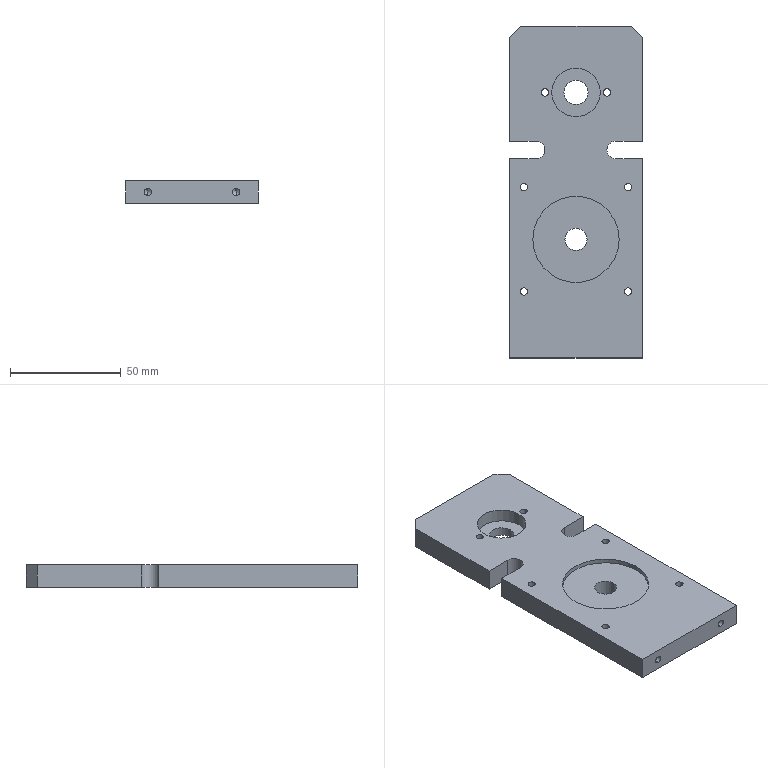Part | SolidWorks | features Cut 4, HoleWzd 3, Chamfer 1, Extrusion 1, ICE 1, MirrorPattern 1 | 1 solid | 47 faces | box 60 x 150 x 10 mm | volume 80933 mm3 | cylinder 27 | plane 16 | cone 4 | commonest cylinder face diameters 3.3 x16 8 x3 10 x2 11 x2 22 x2 39 x2
STEP:
#1=CARTESIAN_POINT('',(20.,-63.5,6.65));
#2=VERTEX_POINT('',#1);
#3=CARTESIAN_POINT('',(20.,-63.5,3.35));
#4=VERTEX_POINT('',#3);
#5=CARTESIAN_POINT('',(20.,-63.5,5.));
#6=DIRECTION('',(0.,-1.,0.));
#7=DIRECTION('',(0.,0.,-1.));
#8=AXIS2_PLACEMENT_3D('',#5,#6,#7);
#9=CIRCLE('',#8,1.65);
#10=EDGE_CURVE('',#2,#4,#9,.T.);
#11=ORIENTED_EDGE('',*,*,#10,.F.);
#12=CARTESIAN_POINT('',(20.,-75.,6.65));
#13=VERTEX_POINT('',#12);
#14=CARTESIAN_POINT('',(20.,-75.,6.65));
#15=DIRECTION('',(0.,-1.,0.));
#16=VECTOR('',#15,1000.);
#17=LINE('',#14,#16);
#18=EDGE_CURVE('',#2,#13,#17,.T.);
#19=ORIENTED_EDGE('',*,*,#18,.T.);
#20=CARTESIAN_POINT('',(20.,-75.,3.35));
#21=VERTEX_POINT('',#20);
#22=CARTESIAN_POINT('',(20.,-75.,5.));
#23=DIRECTION('',(0.,-1.,0.));
#24=DIRECTION('',(0.,0.,-1.));
#25=AXIS2_PLACEMENT_3D('',#22,#23,#24);
#26=CIRCLE('',#25,1.65);
#27=EDGE_CURVE('',#13,#21,#26,.T.);
#28=ORIENTED_EDGE('',*,*,#27,.T.);
#29=CARTESIAN_POINT('',(20.,-75.,3.35));
#30=DIRECTION('',(0.,-1.,0.));
#31=VECTOR('',#30,1000.);
#32=LINE('',#29,#31);
#33=EDGE_CURVE('',#4,#21,#32,.T.);
#34=ORIENTED_EDGE('',*,*,#33,.F.);
#35=EDGE_LOOP('',(#11,#19,#28,#34));
#36=FACE_OUTER_BOUND('',#35,.T.);
#37=CARTESIAN_POINT('',(20.,-75.,5.));
#38=DIRECTION('',(0.,-1.,0.));
#39=DIRECTION('',(0.,0.,-1.));
#40=AXIS2_PLACEMENT_3D('',#37,#38,#39);
#41=CYLINDRICAL_SURFACE('',#40,1.65);
#42=ADVANCED_FACE('',(#36),#41,.F.);
#43=CARTESIAN_POINT('',(20.,-62.509,5.));
#44=VERTEX_POINT('',#43);
#45=CARTESIAN_POINT('',(20.,-63.5,3.35));
#46=DIRECTION('',(0.,-0.515,-0.8572));
#47=VECTOR('',#46,1000.);
#48=LINE('',#45,#47);
#49=EDGE_CURVE('',#44,#4,#48,.T.);
#50=ORIENTED_EDGE('',*,*,#49,.F.);
#51=CARTESIAN_POINT('',(20.,-63.5,6.65));
#52=DIRECTION('',(0.,-0.515,0.8572));
#53=VECTOR('',#52,1000.);
#54=LINE('',#51,#53);
#55=EDGE_CURVE('',#44,#2,#54,.T.);
#56=ORIENTED_EDGE('',*,*,#55,.T.);
#57=ORIENTED_EDGE('',*,*,#10,.T.);
#58=EDGE_LOOP('',(#50,#56,#57));
#59=FACE_OUTER_BOUND('',#58,.T.);
#60=CARTESIAN_POINT('',(20.,-63.5,5.));
#61=DIRECTION('',(0.,-1.,0.));
#62=DIRECTION('',(0.,0.,-1.));
#63=AXIS2_PLACEMENT_3D('',#60,#61,#62);
#64=CONICAL_SURFACE('',#63,1.65,1.03);
#65=ADVANCED_FACE('',(#59),#64,.F.);
#66=CARTESIAN_POINT('',(-20.,-63.5,6.65));
#67=VERTEX_POINT('',#66);
#68=CARTESIAN_POINT('',(-20.,-63.5,3.35));
#69=VERTEX_POINT('',#68);
#70=CARTESIAN_POINT('',(-20.,-63.5,5.));
#71=DIRECTION('',(0.,-1.,0.));
#72=DIRECTION('',(0.,0.,-1.));
#73=AXIS2_PLACEMENT_3D('',#70,#71,#72);
#74=CIRCLE('',#73,1.65);
#75=EDGE_CURVE('',#67,#69,#74,.T.);
#76=ORIENTED_EDGE('',*,*,#75,.F.);
#77=CARTESIAN_POINT('',(-20.,-75.,6.65));
#78=VERTEX_POINT('',#77);
#79=CARTESIAN_POINT('',(-20.,-75.,6.65));
#80=DIRECTION('',(0.,-1.,0.));
#81=VECTOR('',#80,1000.);
#82=LINE('',#79,#81);
#83=EDGE_CURVE('',#67,#78,#82,.T.);
#84=ORIENTED_EDGE('',*,*,#83,.T.);
#85=CARTESIAN_POINT('',(-20.,-75.,3.35));
#86=VERTEX_POINT('',#85);
#87=CARTESIAN_POINT('',(-20.,-75.,5.));
#88=DIRECTION('',(0.,-1.,0.));
#89=DIRECTION('',(0.,0.,-1.));
#90=AXIS2_PLACEMENT_3D('',#87,#88,#89);
#91=CIRCLE('',#90,1.65);
#92=EDGE_CURVE('',#78,#86,#91,.T.);
#93=ORIENTED_EDGE('',*,*,#92,.T.);
#94=CARTESIAN_POINT('',(-20.,-75.,3.35));
#95=DIRECTION('',(0.,-1.,0.));
#96=VECTOR('',#95,1000.);
#97=LINE('',#94,#96);
#98=EDGE_CURVE('',#69,#86,#97,.T.);
#99=ORIENTED_EDGE('',*,*,#98,.F.);
#100=EDGE_LOOP('',(#76,#84,#93,#99));
#101=FACE_OUTER_BOUND('',#100,.T.);
#102=CARTESIAN_POINT('',(-20.,-75.,5.));
#103=DIRECTION('',(0.,-1.,0.));
#104=DIRECTION('',(0.,0.,-1.));
#105=AXIS2_PLACEMENT_3D('',#102,#103,#104);
#106=CYLINDRICAL_SURFACE('',#105,1.65);
#107=ADVANCED_FACE('',(#101),#106,.F.);
#108=CARTESIAN_POINT('',(-20.,-62.509,5.));
#109=VERTEX_POINT('',#108);
#110=CARTESIAN_POINT('',(-20.,-63.5,3.35));
#111=DIRECTION('',(0.,-0.515,-0.8572));
#112=VECTOR('',#111,1000.);
#113=LINE('',#110,#112);
#114=EDGE_CURVE('',#109,#69,#113,.T.);
#115=ORIENTED_EDGE('',*,*,#114,.F.);
#116=CARTESIAN_POINT('',(-20.,-63.5,6.65));
#117=DIRECTION('',(0.,-0.515,0.8572));
#118=VECTOR('',#117,1000.);
#119=LINE('',#116,#118);
#120=EDGE_CURVE('',#109,#67,#119,.T.);
#121=ORIENTED_EDGE('',*,*,#120,.T.);
#122=ORIENTED_EDGE('',*,*,#75,.T.);
#123=EDGE_LOOP('',(#115,#121,#122));
#124=FACE_OUTER_BOUND('',#123,.T.);
#125=CARTESIAN_POINT('',(-20.,-63.5,5.));
#126=DIRECTION('',(0.,-1.,0.));
#127=DIRECTION('',(0.,0.,-1.));
#128=AXIS2_PLACEMENT_3D('',#125,#126,#127);
#129=CONICAL_SURFACE('',#128,1.65,1.03);
#130=ADVANCED_FACE('',(#124),#129,.F.);
#131=CARTESIAN_POINT('',(-15.65,45.,0.));
#132=VERTEX_POINT('',#131);
#133=CARTESIAN_POINT('',(-12.35,45.,0.));
#134=VERTEX_POINT('',#133);
#135=CARTESIAN_POINT('',(-14.,45.,0.));
#136=DIRECTION('',(0.,0.,1.));
#137=DIRECTION('',(1.,0.,0.));
#138=AXIS2_PLACEMENT_3D('',#135,#136,#137);
#139=CIRCLE('',#138,1.65);
#140=EDGE_CURVE('',#132,#134,#139,.T.);
#141=ORIENTED_EDGE('',*,*,#140,.F.);
#142=CARTESIAN_POINT('',(-15.65,45.,10.));
#143=VERTEX_POINT('',#142);
#144=CARTESIAN_POINT('',(-15.65,45.,10.));
#145=DIRECTION('',(0.,0.,1.));
#146=VECTOR('',#145,1000.);
#147=LINE('',#144,#146);
#148=EDGE_CURVE('',#132,#143,#147,.T.);
#149=ORIENTED_EDGE('',*,*,#148,.T.);
#150=CARTESIAN_POINT('',(-12.35,45.,10.));
#151=VERTEX_POINT('',#150);
#152=CARTESIAN_POINT('',(-14.,45.,10.));
#153=DIRECTION('',(0.,0.,1.));
#154=DIRECTION('',(1.,0.,0.));
#155=AXIS2_PLACEMENT_3D('',#152,#153,#154);
#156=CIRCLE('',#155,1.65);
#157=EDGE_CURVE('',#143,#151,#156,.T.);
#158=ORIENTED_EDGE('',*,*,#157,.T.);
#159=CARTESIAN_POINT('',(-12.35,45.,10.));
#160=DIRECTION('',(0.,0.,1.));
#161=VECTOR('',#160,1000.);
#162=LINE('',#159,#161);
#163=EDGE_CURVE('',#134,#151,#162,.T.);
#164=ORIENTED_EDGE('',*,*,#163,.F.);
#165=EDGE_LOOP('',(#141,#149,#158,#164));
#166=FACE_OUTER_BOUND('',#165,.T.);
#167=CARTESIAN_POINT('',(-14.,45.,10.));
#168=DIRECTION('',(0.,0.,1.));
#169=DIRECTION('',(1.,0.,0.));
#170=AXIS2_PLACEMENT_3D('',#167,#168,#169);
#171=CYLINDRICAL_SURFACE('',#170,1.65);
#172=ADVANCED_FACE('',(#166),#171,.F.);
#173=CARTESIAN_POINT('',(12.35,45.,0.));
#174=VERTEX_POINT('',#173);
#175=CARTESIAN_POINT('',(15.65,45.,0.));
#176=VERTEX_POINT('',#175);
#177=CARTESIAN_POINT('',(14.,45.,0.));
#178=DIRECTION('',(0.,0.,1.));
#179=DIRECTION('',(1.,0.,0.));
#180=AXIS2_PLACEMENT_3D('',#177,#178,#179);
#181=CIRCLE('',#180,1.65);
#182=EDGE_CURVE('',#174,#176,#181,.T.);
#183=ORIENTED_EDGE('',*,*,#182,.F.);
#184=CARTESIAN_POINT('',(12.35,45.,10.));
#185=VERTEX_POINT('',#184);
#186=CARTESIAN_POINT('',(12.35,45.,10.));
#187=DIRECTION('',(0.,0.,1.));
#188=VECTOR('',#187,1000.);
#189=LINE('',#186,#188);
#190=EDGE_CURVE('',#174,#185,#189,.T.);
#191=ORIENTED_EDGE('',*,*,#190,.T.);
#192=CARTESIAN_POINT('',(15.65,45.,10.));
#193=VERTEX_POINT('',#192);
#194=CARTESIAN_POINT('',(14.,45.,10.));
#195=DIRECTION('',(0.,0.,1.));
#196=DIRECTION('',(1.,0.,0.));
#197=AXIS2_PLACEMENT_3D('',#194,#195,#196);
#198=CIRCLE('',#197,1.65);
#199=EDGE_CURVE('',#185,#193,#198,.T.);
#200=ORIENTED_EDGE('',*,*,#199,.T.);
#201=CARTESIAN_POINT('',(15.65,45.,10.));
#202=DIRECTION('',(0.,0.,1.));
#203=VECTOR('',#202,1000.);
#204=LINE('',#201,#203);
#205=EDGE_CURVE('',#176,#193,#204,.T.);
#206=ORIENTED_EDGE('',*,*,#205,.F.);
#207=EDGE_LOOP('',(#183,#191,#200,#206));
#208=FACE_OUTER_BOUND('',#207,.T.);
#209=CARTESIAN_POINT('',(14.,45.,10.));
#210=DIRECTION('',(0.,0.,1.));
#211=DIRECTION('',(1.,0.,0.));
#212=AXIS2_PLACEMENT_3D('',#209,#210,#211);
#213=CYLINDRICAL_SURFACE('',#212,1.65);
#214=ADVANCED_FACE('',(#208),#213,.F.);
#215=CARTESIAN_POINT('',(18.,23.,10.));
#216=VERTEX_POINT('',#215);
#217=CARTESIAN_POINT('',(14.,19.,10.));
#218=VERTEX_POINT('',#217);
#219=CARTESIAN_POINT('',(18.,19.,10.));
#220=DIRECTION('',(0.,0.,1.));
#221=DIRECTION('',(1.,0.,0.));
#222=AXIS2_PLACEMENT_3D('',#219,#220,#221);
#223=CIRCLE('',#222,4.);
#224=EDGE_CURVE('',#216,#218,#223,.T.);
#225=ORIENTED_EDGE('',*,*,#224,.T.);
#226=CARTESIAN_POINT('',(14.,19.,0.));
#227=VERTEX_POINT('',#226);
#228=CARTESIAN_POINT('',(14.,19.,10.));
#229=DIRECTION('',(0.,0.,-1.));
#230=VECTOR('',#229,1000.);
#231=LINE('',#228,#230);
#232=EDGE_CURVE('',#218,#227,#231,.T.);
#233=ORIENTED_EDGE('',*,*,#232,.T.);
#234=CARTESIAN_POINT('',(18.,23.,0.));
#235=VERTEX_POINT('',#234);
#236=CARTESIAN_POINT('',(18.,19.,0.));
#237=DIRECTION('',(0.,0.,1.));
#238=DIRECTION('',(1.,0.,0.));
#239=AXIS2_PLACEMENT_3D('',#236,#237,#238);
#240=CIRCLE('',#239,4.);
#241=EDGE_CURVE('',#235,#227,#240,.T.);
#242=ORIENTED_EDGE('',*,*,#241,.F.);
#243=CARTESIAN_POINT('',(18.,23.,10.));
#244=DIRECTION('',(0.,0.,-1.));
#245=VECTOR('',#244,1000.);
#246=LINE('',#243,#245);
#247=EDGE_CURVE('',#216,#235,#246,.T.);
#248=ORIENTED_EDGE('',*,*,#247,.F.);
#249=EDGE_LOOP('',(#225,#233,#242,#248));
#250=FACE_OUTER_BOUND('',#249,.T.);
#251=CARTESIAN_POINT('',(18.,19.,10.));
#252=DIRECTION('',(0.,0.,-1.));
#253=DIRECTION('',(-1.,0.,0.));
#254=AXIS2_PLACEMENT_3D('',#251,#252,#253);
#255=CYLINDRICAL_SURFACE('',#254,4.);
#256=ADVANCED_FACE('',(#250),#255,.F.);
#257=CARTESIAN_POINT('',(-5.5,45.,0.));
#258=VERTEX_POINT('',#257);
#259=CARTESIAN_POINT('',(5.5,45.,0.));
#260=VERTEX_POINT('',#259);
#261=CARTESIAN_POINT('',(0.,45.,0.));
#262=DIRECTION('',(0.,0.,1.));
#263=DIRECTION('',(1.,0.,0.));
#264=AXIS2_PLACEMENT_3D('',#261,#262,#263);
#265=CIRCLE('',#264,5.5);
#266=EDGE_CURVE('',#258,#260,#265,.T.);
#267=ORIENTED_EDGE('',*,*,#266,.F.);
#268=CARTESIAN_POINT('',(-5.5,45.,4.));
#269=VERTEX_POINT('',#268);
#270=CARTESIAN_POINT('',(-5.5,45.,0.));
#271=DIRECTION('',(0.,0.,1.));
#272=VECTOR('',#271,1000.);
#273=LINE('',#270,#272);
#274=EDGE_CURVE('',#258,#269,#273,.T.);
#275=ORIENTED_EDGE('',*,*,#274,.T.);
#276=CARTESIAN_POINT('',(5.5,45.,4.));
#277=VERTEX_POINT('',#276);
#278=CARTESIAN_POINT('',(0.,45.,4.));
#279=DIRECTION('',(0.,0.,1.));
#280=DIRECTION('',(1.,0.,0.));
#281=AXIS2_PLACEMENT_3D('',#278,#279,#280);
#282=CIRCLE('',#281,5.5);
#283=EDGE_CURVE('',#269,#277,#282,.T.);
#284=ORIENTED_EDGE('',*,*,#283,.T.);
#285=CARTESIAN_POINT('',(5.5,45.,0.));
#286=DIRECTION('',(0.,0.,1.));
#287=VECTOR('',#286,1000.);
#288=LINE('',#285,#287);
#289=EDGE_CURVE('',#260,#277,#288,.T.);
#290=ORIENTED_EDGE('',*,*,#289,.F.);
#291=EDGE_LOOP('',(#267,#275,#284,#290));
#292=FACE_OUTER_BOUND('',#291,.T.);
#293=CARTESIAN_POINT('',(0.,45.,0.));
#294=DIRECTION('',(0.,0.,1.));
#295=DIRECTION('',(1.,0.,0.));
#296=AXIS2_PLACEMENT_3D('',#293,#294,#295);
#297=CYLINDRICAL_SURFACE('',#296,5.5);
#298=ADVANCED_FACE('',(#292),#297,.F.);
#299=CARTESIAN_POINT('',(-11.,45.,4.));
#300=VERTEX_POINT('',#299);
#301=CARTESIAN_POINT('',(11.,45.,4.));
#302=VERTEX_POINT('',#301);
#303=CARTESIAN_POINT('',(0.,45.,4.));
#304=DIRECTION('',(0.,0.,1.));
#305=DIRECTION('',(1.,0.,0.));
#306=AXIS2_PLACEMENT_3D('',#303,#304,#305);
#307=CIRCLE('',#306,11.);
#308=EDGE_CURVE('',#300,#302,#307,.T.);
#309=ORIENTED_EDGE('',*,*,#308,.F.);
#310=CARTESIAN_POINT('',(-11.,45.,10.));
#311=VERTEX_POINT('',#310);
#312=CARTESIAN_POINT('',(-11.,45.,4.));
#313=DIRECTION('',(0.,0.,1.));
#314=VECTOR('',#313,1000.);
#315=LINE('',#312,#314);
#316=EDGE_CURVE('',#300,#311,#315,.T.);
#317=ORIENTED_EDGE('',*,*,#316,.T.);
#318=CARTESIAN_POINT('',(11.,45.,10.));
#319=VERTEX_POINT('',#318);
#320=CARTESIAN_POINT('',(0.,45.,10.));
#321=DIRECTION('',(0.,0.,1.));
#322=DIRECTION('',(1.,0.,0.));
#323=AXIS2_PLACEMENT_3D('',#320,#321,#322);
#324=CIRCLE('',#323,11.);
#325=EDGE_CURVE('',#311,#319,#324,.T.);
#326=ORIENTED_EDGE('',*,*,#325,.T.);
#327=CARTESIAN_POINT('',(11.,45.,4.));
#328=DIRECTION('',(0.,0.,1.));
#329=VECTOR('',#328,1000.);
#330=LINE('',#327,#329);
#331=EDGE_CURVE('',#302,#319,#330,.T.);
#332=ORIENTED_EDGE('',*,*,#331,.F.);
#333=EDGE_LOOP('',(#309,#317,#326,#332));
#334=FACE_OUTER_BOUND('',#333,.T.);
#335=CARTESIAN_POINT('',(0.,45.,4.));
#336=DIRECTION('',(0.,0.,1.));
#337=DIRECTION('',(1.,0.,0.));
#338=AXIS2_PLACEMENT_3D('',#335,#336,#337);
#339=CYLINDRICAL_SURFACE('',#338,11.);
#340=ADVANCED_FACE('',(#334),#339,.F.);
#341=CARTESIAN_POINT('',(-25.22,2.145,0.));
#342=VERTEX_POINT('',#341);
#343=CARTESIAN_POINT('',(-21.92,2.145,0.));
#344=VERTEX_POINT('',#343);
#345=CARTESIAN_POINT('',(-23.57,2.145,0.));
#346=DIRECTION('',(0.,0.,1.));
#347=DIRECTION('',(1.,0.,0.));
#348=AXIS2_PLACEMENT_3D('',#345,#346,#347);
#349=CIRCLE('',#348,1.65);
#350=EDGE_CURVE('',#342,#344,#349,.T.);
#351=ORIENTED_EDGE('',*,*,#350,.F.);
#352=CARTESIAN_POINT('',(-25.22,2.145,10.));
#353=VERTEX_POINT('',#352);
#354=CARTESIAN_POINT('',(-25.22,2.145,10.));
#355=DIRECTION('',(0.,0.,1.));
#356=VECTOR('',#355,1000.);
#357=LINE('',#354,#356);
#358=EDGE_CURVE('',#342,#353,#357,.T.);
#359=ORIENTED_EDGE('',*,*,#358,.T.);
#360=CARTESIAN_POINT('',(-21.92,2.145,10.));
#361=VERTEX_POINT('',#360);
#362=CARTESIAN_POINT('',(-23.57,2.145,10.));
#363=DIRECTION('',(0.,0.,1.));
#364=DIRECTION('',(1.,0.,0.));
#365=AXIS2_PLACEMENT_3D('',#362,#363,#364);
#366=CIRCLE('',#365,1.65);
#367=EDGE_CURVE('',#353,#361,#366,.T.);
#368=ORIENTED_EDGE('',*,*,#367,.T.);
#369=CARTESIAN_POINT('',(-21.92,2.145,10.));
#370=DIRECTION('',(0.,0.,1.));
#371=VECTOR('',#370,1000.);
#372=LINE('',#369,#371);
#373=EDGE_CURVE('',#344,#361,#372,.T.);
#374=ORIENTED_EDGE('',*,*,#373,.F.);
#375=EDGE_LOOP('',(#351,#359,#368,#374));
#376=FACE_OUTER_BOUND('',#375,.T.);
#377=CARTESIAN_POINT('',(-23.57,2.145,10.));
#378=DIRECTION('',(0.,0.,1.));
#379=DIRECTION('',(1.,0.,0.));
#380=AXIS2_PLACEMENT_3D('',#377,#378,#379);
#381=CYLINDRICAL_SURFACE('',#380,1.65);
#382=ADVANCED_FACE('',(#376),#381,.F.);
#383=CARTESIAN_POINT('',(-25.22,-44.995,0.));
#384=VERTEX_POINT('',#383);
#385=CARTESIAN_POINT('',(-21.92,-44.995,0.));
#386=VERTEX_POINT('',#385);
#387=CARTESIAN_POINT('',(-23.57,-44.995,0.));
#388=DIRECTION('',(0.,0.,1.));
#389=DIRECTION('',(1.,0.,0.));
#390=AXIS2_PLACEMENT_3D('',#387,#388,#389);
#391=CIRCLE('',#390,1.65);
#392=EDGE_CURVE('',#384,#386,#391,.T.);
#393=ORIENTED_EDGE('',*,*,#392,.F.);
#394=CARTESIAN_POINT('',(-25.22,-44.995,10.));
#395=VERTEX_POINT('',#394);
#396=CARTESIAN_POINT('',(-25.22,-44.995,10.));
#397=DIRECTION('',(0.,0.,1.));
#398=VECTOR('',#397,1000.);
#399=LINE('',#396,#398);
#400=EDGE_CURVE('',#384,#395,#399,.T.);
#401=ORIENTED_EDGE('',*,*,#400,.T.);
#402=CARTESIAN_POINT('',(-21.92,-44.995,10.));
#403=VERTEX_POINT('',#402);
#404=CARTESIAN_POINT('',(-23.57,-44.995,10.));
#405=DIRECTION('',(0.,0.,1.));
#406=DIRECTION('',(1.,0.,0.));
#407=AXIS2_PLACEMENT_3D('',#404,#405,#406);
#408=CIRCLE('',#407,1.65);
#409=EDGE_CURVE('',#395,#403,#408,.T.);
#410=ORIENTED_EDGE('',*,*,#409,.T.);
#411=CARTESIAN_POINT('',(-21.92,-44.995,10.));
#412=DIRECTION('',(0.,0.,1.));
#413=VECTOR('',#412,1000.);
#414=LINE('',#411,#413);
#415=EDGE_CURVE('',#386,#403,#414,.T.);
#416=ORIENTED_EDGE('',*,*,#415,.F.);
#417=EDGE_LOOP('',(#393,#401,#410,#416));
#418=FACE_OUTER_BOUND('',#417,.T.);
#419=CARTESIAN_POINT('',(-23.57,-44.995,10.));
#420=DIRECTION('',(0.,0.,1.));
#421=DIRECTION('',(1.,0.,0.));
#422=AXIS2_PLACEMENT_3D('',#419,#420,#421);
#423=CYLINDRICAL_SURFACE('',#422,1.65);
#424=ADVANCED_FACE('',(#418),#423,.F.);
#425=CARTESIAN_POINT('',(21.92,2.145,0.));
#426=VERTEX_POINT('',#425);
#427=CARTESIAN_POINT('',(25.22,2.145,0.));
#428=VERTEX_POINT('',#427);
#429=CARTESIAN_POINT('',(23.57,2.145,0.));
#430=DIRECTION('',(0.,0.,1.));
#431=DIRECTION('',(1.,0.,0.));
#432=AXIS2_PLACEMENT_3D('',#429,#430,#431);
#433=CIRCLE('',#432,1.65);
#434=EDGE_CURVE('',#426,#428,#433,.T.);
#435=ORIENTED_EDGE('',*,*,#434,.F.);
#436=CARTESIAN_POINT('',(21.92,2.145,10.));
#437=VERTEX_POINT('',#436);
#438=CARTESIAN_POINT('',(21.92,2.145,10.));
#439=DIRECTION('',(0.,0.,1.));
#440=VECTOR('',#439,1000.);
#441=LINE('',#438,#440);
#442=EDGE_CURVE('',#426,#437,#441,.T.);
#443=ORIENTED_EDGE('',*,*,#442,.T.);
#444=CARTESIAN_POINT('',(25.22,2.145,10.));
#445=VERTEX_POINT('',#444);
#446=CARTESIAN_POINT('',(23.57,2.145,10.));
#447=DIRECTION('',(0.,0.,1.));
#448=DIRECTION('',(1.,0.,0.));
#449=AXIS2_PLACEMENT_3D('',#446,#447,#448);
#450=CIRCLE('',#449,1.65);
#451=EDGE_CURVE('',#437,#445,#450,.T.);
#452=ORIENTED_EDGE('',*,*,#451,.T.);
#453=CARTESIAN_POINT('',(25.22,2.145,10.));
#454=DIRECTION('',(0.,0.,1.));
#455=VECTOR('',#454,1000.);
#456=LINE('',#453,#455);
#457=EDGE_CURVE('',#428,#445,#456,.T.);
#458=ORIENTED_EDGE('',*,*,#457,.F.);
#459=EDGE_LOOP('',(#435,#443,#452,#458));
#460=FACE_OUTER_BOUND('',#459,.T.);
#461=CARTESIAN_POINT('',(23.57,2.145,10.));
#462=DIRECTION('',(0.,0.,1.));
#463=DIRECTION('',(1.,0.,0.));
#464=AXIS2_PLACEMENT_3D('',#461,#462,#463);
#465=CYLINDRICAL_SURFACE('',#464,1.65);
#466=ADVANCED_FACE('',(#460),#465,.F.);
#467=CARTESIAN_POINT('',(21.92,-44.995,0.));
#468=VERTEX_POINT('',#467);
#469=CARTESIAN_POINT('',(25.22,-44.995,0.));
#470=VERTEX_POINT('',#469);
#471=CARTESIAN_POINT('',(23.57,-44.995,0.));
#472=DIRECTION('',(0.,0.,1.));
#473=DIRECTION('',(1.,0.,0.));
#474=AXIS2_PLACEMENT_3D('',#471,#472,#473);
#475=CIRCLE('',#474,1.65);
#476=EDGE_CURVE('',#468,#470,#475,.T.);
#477=ORIENTED_EDGE('',*,*,#476,.F.);
#478=CARTESIAN_POINT('',(21.92,-44.995,10.));
#479=VERTEX_POINT('',#478);
#480=CARTESIAN_POINT('',(21.92,-44.995,10.));
#481=DIRECTION('',(0.,0.,1.));
#482=VECTOR('',#481,1000.);
#483=LINE('',#480,#482);
#484=EDGE_CURVE('',#468,#479,#483,.T.);
#485=ORIENTED_EDGE('',*,*,#484,.T.);
#486=CARTESIAN_POINT('',(25.22,-44.995,10.));
#487=VERTEX_POINT('',#486);
#488=CARTESIAN_POINT('',(23.57,-44.995,10.));
#489=DIRECTION('',(0.,0.,1.));
#490=DIRECTION('',(1.,0.,0.));
#491=AXIS2_PLACEMENT_3D('',#488,#489,#490);
#492=CIRCLE('',#491,1.65);
#493=EDGE_CURVE('',#479,#487,#492,.T.);
#494=ORIENTED_EDGE('',*,*,#493,.T.);
#495=CARTESIAN_POINT('',(25.22,-44.995,10.));
#496=DIRECTION('',(0.,0.,1.));
#497=VECTOR('',#496,1000.);
#498=LINE('',#495,#497);
#499=EDGE_CURVE('',#470,#487,#498,.T.);
#500=ORIENTED_EDGE('',*,*,#499,.F.);
#501=EDGE_LOOP('',(#477,#485,#494,#500));
#502=FACE_OUTER_BOUND('',#501,.T.);
#503=CARTESIAN_POINT('',(23.57,-44.995,10.));
#504=DIRECTION('',(0.,0.,1.));
#505=DIRECTION('',(1.,0.,0.));
#506=AXIS2_PLACEMENT_3D('',#503,#504,#505);
#507=CYLINDRICAL_SURFACE('',#506,1.65);
#508=ADVANCED_FACE('',(#502),#507,.F.);
#509=CARTESIAN_POINT('',(-5.,-21.425,0.));
#510=VERTEX_POINT('',#509);
#511=CARTESIAN_POINT('',(5.,-21.425,0.));
#512=VERTEX_POINT('',#511);
#513=CARTESIAN_POINT('',(0.,-21.425,0.));
#514=DIRECTION('',(0.,0.,1.));
#515=DIRECTION('',(1.,0.,0.));
#516=AXIS2_PLACEMENT_3D('',#513,#514,#515);
#517=CIRCLE('',#516,5.);
#518=EDGE_CURVE('',#510,#512,#517,.T.);
#519=ORIENTED_EDGE('',*,*,#518,.F.);
#520=CARTESIAN_POINT('',(-5.,-21.425,8.));
#521=VERTEX_POINT('',#520);
#522=CARTESIAN_POINT('',(-5.,-21.425,0.));
#523=DIRECTION('',(0.,0.,1.));
#524=VECTOR('',#523,1000.);
#525=LINE('',#522,#524);
#526=EDGE_CURVE('',#510,#521,#525,.T.);
#527=ORIENTED_EDGE('',*,*,#526,.T.);
#528=CARTESIAN_POINT('',(5.,-21.425,8.));
#529=VERTEX_POINT('',#528);
#530=CARTESIAN_POINT('',(0.,-21.425,8.));
#531=DIRECTION('',(0.,0.,1.));
#532=DIRECTION('',(1.,0.,0.));
#533=AXIS2_PLACEMENT_3D('',#530,#531,#532);
#534=CIRCLE('',#533,5.);
#535=EDGE_CURVE('',#521,#529,#534,.T.);
#536=ORIENTED_EDGE('',*,*,#535,.T.);
#537=CARTESIAN_POINT('',(5.,-21.425,0.));
#538=DIRECTION('',(0.,0.,1.));
#539=VECTOR('',#538,1000.);
#540=LINE('',#537,#539);
#541=EDGE_CURVE('',#512,#529,#540,.T.);
#542=ORIENTED_EDGE('',*,*,#541,.F.);
#543=EDGE_LOOP('',(#519,#527,#536,#542));
#544=FACE_OUTER_BOUND('',#543,.T.);
#545=CARTESIAN_POINT('',(0.,-21.425,0.));
#546=DIRECTION('',(0.,0.,1.));
#547=DIRECTION('',(1.,0.,0.));
#548=AXIS2_PLACEMENT_3D('',#545,#546,#547);
#549=CYLINDRICAL_SURFACE('',#548,5.);
#550=ADVANCED_FACE('',(#544),#549,.F.);
#551=CARTESIAN_POINT('',(19.5,-21.425,8.));
#552=VERTEX_POINT('',#551);
#553=CARTESIAN_POINT('',(-19.5,-21.425,8.));
#554=VERTEX_POINT('',#553);
#555=CARTESIAN_POINT('',(0.,-21.425,8.));
#556=DIRECTION('',(0.,0.,-1.));
#557=DIRECTION('',(-1.,0.,0.));
#558=AXIS2_PLACEMENT_3D('',#555,#556,#557);
#559=CIRCLE('',#558,19.5);
#560=EDGE_CURVE('',#552,#554,#559,.T.);
#561=ORIENTED_EDGE('',*,*,#560,.T.);
#562=CARTESIAN_POINT('',(-19.5,-21.425,10.));
#563=VERTEX_POINT('',#562);
#564=CARTESIAN_POINT('',(-19.5,-21.425,8.));
#565=DIRECTION('',(0.,0.,1.));
#566=VECTOR('',#565,1000.);
#567=LINE('',#564,#566);
#568=EDGE_CURVE('',#554,#563,#567,.T.);
#569=ORIENTED_EDGE('',*,*,#568,.T.);
#570=CARTESIAN_POINT('',(19.5,-21.425,10.));
#571=VERTEX_POINT('',#570);
#572=CARTESIAN_POINT('',(0.,-21.425,10.));
#573=DIRECTION('',(0.,0.,-1.));
#574=DIRECTION('',(-1.,0.,0.));
#575=AXIS2_PLACEMENT_3D('',#572,#573,#574);
#576=CIRCLE('',#575,19.5);
#577=EDGE_CURVE('',#571,#563,#576,.T.);
#578=ORIENTED_EDGE('',*,*,#577,.F.);
#579=CARTESIAN_POINT('',(19.5,-21.425,8.));
#580=DIRECTION('',(0.,0.,1.));
#581=VECTOR('',#580,1000.);
#582=LINE('',#579,#581);
#583=EDGE_CURVE('',#552,#571,#582,.T.);
#584=ORIENTED_EDGE('',*,*,#583,.F.);
#585=EDGE_LOOP('',(#561,#569,#578,#584));
#586=FACE_OUTER_BOUND('',#585,.T.);
#587=CARTESIAN_POINT('',(0.,-21.425,8.));
#588=DIRECTION('',(0.,0.,1.));
#589=DIRECTION('',(1.,0.,0.));
#590=AXIS2_PLACEMENT_3D('',#587,#588,#589);
#591=CYLINDRICAL_SURFACE('',#590,19.5);
#592=ADVANCED_FACE('',(#586),#591,.F.);
#593=CARTESIAN_POINT('',(30.,15.,10.));
#594=VERTEX_POINT('',#593);
#595=CARTESIAN_POINT('',(30.,15.,0.));
#596=VERTEX_POINT('',#595);
#597=CARTESIAN_POINT('',(30.,15.,10.));
#598=DIRECTION('',(0.,0.,-1.));
#599=VECTOR('',#598,1000.);
#600=LINE('',#597,#599);
#601=EDGE_CURVE('',#594,#596,#600,.T.);
#602=ORIENTED_EDGE('',*,*,#601,.F.);
#603=CARTESIAN_POINT('',(30.,-75.,10.));
#604=VERTEX_POINT('',#603);
#605=CARTESIAN_POINT('',(30.,75.,10.));
#606=DIRECTION('',(0.,1.,0.));
#607=VECTOR('',#606,1000.);
#608=LINE('',#605,#607);
#609=EDGE_CURVE('',#604,#594,#608,.T.);
#610=ORIENTED_EDGE('',*,*,#609,.F.);
#611=CARTESIAN_POINT('',(30.,-75.,0.));
#612=VERTEX_POINT('',#611);
#613=CARTESIAN_POINT('',(30.,-75.,10.));
#614=DIRECTION('',(0.,0.,-1.));
#615=VECTOR('',#614,1000.);
#616=LINE('',#613,#615);
#617=EDGE_CURVE('',#604,#612,#616,.T.);
#618=ORIENTED_EDGE('',*,*,#617,.T.);
#619=CARTESIAN_POINT('',(30.,75.,0.));
#620=DIRECTION('',(0.,1.,0.));
#621=VECTOR('',#620,1000.);
#622=LINE('',#619,#621);
#623=EDGE_CURVE('',#612,#596,#622,.T.);
#624=ORIENTED_EDGE('',*,*,#623,.T.);
#625=EDGE_LOOP('',(#602,#610,#618,#624));
#626=FACE_OUTER_BOUND('',#625,.T.);
#627=CARTESIAN_POINT('',(30.,75.,10.));
#628=DIRECTION('',(-1.,0.,0.));
#629=DIRECTION('',(0.,-1.,0.));
#630=AXIS2_PLACEMENT_3D('',#627,#628,#629);
#631=PLANE('',#630);
#632=ADVANCED_FACE('',(#626),#631,.F.);
#633=CARTESIAN_POINT('',(30.,23.,0.));
#634=VERTEX_POINT('',#633);
#635=CARTESIAN_POINT('',(30.,23.,10.));
#636=VERTEX_POINT('',#635);
#637=CARTESIAN_POINT('',(30.,23.,10.));
#638=DIRECTION('',(0.,0.,1.));
#639=VECTOR('',#638,1000.);
#640=LINE('',#637,#639);
#641=EDGE_CURVE('',#634,#636,#640,.T.);
#642=ORIENTED_EDGE('',*,*,#641,.F.);
#643=CARTESIAN_POINT('',(30.,70.,0.));
#644=VERTEX_POINT('',#643);
#645=CARTESIAN_POINT('',(30.,75.,0.));
#646=DIRECTION('',(0.,1.,0.));
#647=VECTOR('',#646,1000.);
#648=LINE('',#645,#647);
#649=EDGE_CURVE('',#634,#644,#648,.T.);
#650=ORIENTED_EDGE('',*,*,#649,.T.);
#651=CARTESIAN_POINT('',(30.,70.,10.));
#652=VERTEX_POINT('',#651);
#653=CARTESIAN_POINT('',(30.,70.,10.));
#654=DIRECTION('',(0.,0.,1.));
#655=VECTOR('',#654,1000.);
#656=LINE('',#653,#655);
#657=EDGE_CURVE('',#644,#652,#656,.T.);
#658=ORIENTED_EDGE('',*,*,#657,.T.);
#659=CARTESIAN_POINT('',(30.,75.,10.));
#660=DIRECTION('',(0.,1.,0.));
#661=VECTOR('',#660,1000.);
#662=LINE('',#659,#661);
#663=EDGE_CURVE('',#636,#652,#662,.T.);
#664=ORIENTED_EDGE('',*,*,#663,.F.);
#665=EDGE_LOOP('',(#642,#650,#658,#664));
#666=FACE_OUTER_BOUND('',#665,.T.);
#667=CARTESIAN_POINT('',(30.,75.,10.));
#668=DIRECTION('',(-1.,0.,0.));
#669=DIRECTION('',(0.,-1.,0.));
#670=AXIS2_PLACEMENT_3D('',#667,#668,#669);
#671=PLANE('',#670);
#672=ADVANCED_FACE('',(#666),#671,.F.);
#673=CARTESIAN_POINT('',(-14.,45.,10.));
#674=DIRECTION('',(0.,0.,1.));
#675=DIRECTION('',(1.,0.,0.));
#676=AXIS2_PLACEMENT_3D('',#673,#674,#675);
#677=CIRCLE('',#676,1.65);
#678=EDGE_CURVE('',#151,#143,#677,.T.);
#679=ORIENTED_EDGE('',*,*,#678,.F.);
#680=ORIENTED_EDGE('',*,*,#157,.F.);
#681=EDGE_LOOP('',(#679,#680));
#682=FACE_BOUND('',#681,.T.);
#683=CARTESIAN_POINT('',(14.,45.,10.));
#684=DIRECTION('',(0.,0.,1.));
#685=DIRECTION('',(1.,0.,0.));
#686=AXIS2_PLACEMENT_3D('',#683,#684,#685);
#687=CIRCLE('',#686,1.65);
#688=EDGE_CURVE('',#193,#185,#687,.T.);
#689=ORIENTED_EDGE('',*,*,#688,.F.);
#690=ORIENTED_EDGE('',*,*,#199,.F.);
#691=EDGE_LOOP('',(#689,#690));
#692=FACE_BOUND('',#691,.T.);
#693=CARTESIAN_POINT('',(0.,45.,10.));
#694=DIRECTION('',(0.,0.,1.));
#695=DIRECTION('',(1.,0.,0.));
#696=AXIS2_PLACEMENT_3D('',#693,#694,#695);
#697=CIRCLE('',#696,11.);
#698=EDGE_CURVE('',#319,#311,#697,.T.);
#699=ORIENTED_EDGE('',*,*,#698,.F.);
#700=ORIENTED_EDGE('',*,*,#325,.F.);
#701=EDGE_LOOP('',(#699,#700));
#702=FACE_BOUND('',#701,.T.);
#703=CARTESIAN_POINT('',(-23.57,2.145,10.));
#704=DIRECTION('',(0.,0.,1.));
#705=DIRECTION('',(1.,0.,0.));
#706=AXIS2_PLACEMENT_3D('',#703,#704,#705);
#707=CIRCLE('',#706,1.65);
#708=EDGE_CURVE('',#361,#353,#707,.T.);
#709=ORIENTED_EDGE('',*,*,#708,.F.);
#710=ORIENTED_EDGE('',*,*,#367,.F.);
#711=EDGE_LOOP('',(#709,#710));
#712=FACE_BOUND('',#711,.T.);
#713=CARTESIAN_POINT('',(-23.57,-44.995,10.));
#714=DIRECTION('',(0.,0.,1.));
#715=DIRECTION('',(1.,0.,0.));
#716=AXIS2_PLACEMENT_3D('',#713,#714,#715);
#717=CIRCLE('',#716,1.65);
#718=EDGE_CURVE('',#403,#395,#717,.T.);
#719=ORIENTED_EDGE('',*,*,#718,.F.);
#720=ORIENTED_EDGE('',*,*,#409,.F.);
#721=EDGE_LOOP('',(#719,#720));
#722=FACE_BOUND('',#721,.T.);
#723=CARTESIAN_POINT('',(23.57,2.145,10.));
#724=DIRECTION('',(0.,0.,1.));
#725=DIRECTION('',(1.,0.,0.));
#726=AXIS2_PLACEMENT_3D('',#723,#724,#725);
#727=CIRCLE('',#726,1.65);
#728=EDGE_CURVE('',#445,#437,#727,.T.);
#729=ORIENTED_EDGE('',*,*,#728,.F.);
#730=ORIENTED_EDGE('',*,*,#451,.F.);
#731=EDGE_LOOP('',(#729,#730));
#732=FACE_BOUND('',#731,.T.);
#733=CARTESIAN_POINT('',(23.57,-44.995,10.));
#734=DIRECTION('',(0.,0.,1.));
#735=DIRECTION('',(1.,0.,0.));
#736=AXIS2_PLACEMENT_3D('',#733,#734,#735);
#737=CIRCLE('',#736,1.65);
#738=EDGE_CURVE('',#487,#479,#737,.T.);
#739=ORIENTED_EDGE('',*,*,#738,.F.);
#740=ORIENTED_EDGE('',*,*,#493,.F.);
#741=EDGE_LOOP('',(#739,#740));
#742=FACE_BOUND('',#741,.T.);
#743=ORIENTED_EDGE('',*,*,#577,.T.);
#744=CARTESIAN_POINT('',(0.,-21.425,10.));
#745=DIRECTION('',(0.,0.,-1.));
#746=DIRECTION('',(-1.,0.,0.));
#747=AXIS2_PLACEMENT_3D('',#744,#745,#746);
#748=CIRCLE('',#747,19.5);
#749=EDGE_CURVE('',#563,#571,#748,.T.);
#750=ORIENTED_EDGE('',*,*,#749,.T.);
#751=EDGE_LOOP('',(#743,#750));
#752=FACE_BOUND('',#751,.T.);
#753=ORIENTED_EDGE('',*,*,#609,.T.);
#754=CARTESIAN_POINT('',(18.,15.,10.));
#755=VERTEX_POINT('',#754);
#756=CARTESIAN_POINT('',(18.,15.,10.));
#757=DIRECTION('',(1.,0.,0.));
#758=VECTOR('',#757,1000.);
#759=LINE('',#756,#758);
#760=EDGE_CURVE('',#755,#594,#759,.T.);
#761=ORIENTED_EDGE('',*,*,#760,.F.);
#762=CARTESIAN_POINT('',(18.,19.,10.));
#763=DIRECTION('',(0.,0.,1.));
#764=DIRECTION('',(1.,0.,0.));
#765=AXIS2_PLACEMENT_3D('',#762,#763,#764);
#766=CIRCLE('',#765,4.);
#767=EDGE_CURVE('',#218,#755,#766,.T.);
#768=ORIENTED_EDGE('',*,*,#767,.F.);
#769=ORIENTED_EDGE('',*,*,#224,.F.);
#770=CARTESIAN_POINT('',(18.,23.,10.));
#771=DIRECTION('',(-1.,0.,0.));
#772=VECTOR('',#771,1000.);
#773=LINE('',#770,#772);
#774=EDGE_CURVE('',#636,#216,#773,.T.);
#775=ORIENTED_EDGE('',*,*,#774,.F.);
#776=ORIENTED_EDGE('',*,*,#663,.T.);
#777=CARTESIAN_POINT('',(25.,75.,10.));
#778=VERTEX_POINT('',#777);
#779=CARTESIAN_POINT('',(50.,50.,10.));
#780=DIRECTION('',(-0.7071,0.7071,0.));
#781=VECTOR('',#780,1000.);
#782=LINE('',#779,#781);
#783=EDGE_CURVE('',#652,#778,#782,.T.);
#784=ORIENTED_EDGE('',*,*,#783,.T.);
#785=CARTESIAN_POINT('',(-25.,75.,10.));
#786=VERTEX_POINT('',#785);
#787=CARTESIAN_POINT('',(-30.,75.,10.));
#788=DIRECTION('',(-1.,0.,0.));
#789=VECTOR('',#788,1000.);
#790=LINE('',#787,#789);
#791=EDGE_CURVE('',#778,#786,#790,.T.);
#792=ORIENTED_EDGE('',*,*,#791,.T.);
#793=CARTESIAN_POINT('',(-30.,70.,10.));
#794=VERTEX_POINT('',#793);
#795=CARTESIAN_POINT('',(-50.,50.,10.));
#796=DIRECTION('',(-0.7071,-0.7071,0.));
#797=VECTOR('',#796,1000.);
#798=LINE('',#795,#797);
#799=EDGE_CURVE('',#786,#794,#798,.T.);
#800=ORIENTED_EDGE('',*,*,#799,.T.);
#801=CARTESIAN_POINT('',(-30.,23.,10.));
#802=VERTEX_POINT('',#801);
#803=CARTESIAN_POINT('',(-30.,75.,10.));
#804=DIRECTION('',(0.,-1.,0.));
#805=VECTOR('',#804,1000.);
#806=LINE('',#803,#805);
#807=EDGE_CURVE('',#794,#802,#806,.T.);
#808=ORIENTED_EDGE('',*,*,#807,.T.);
#809=CARTESIAN_POINT('',(-18.,23.,10.));
#810=VERTEX_POINT('',#809);
#811=CARTESIAN_POINT('',(-18.,23.,10.));
#812=DIRECTION('',(1.,0.,0.));
#813=VECTOR('',#812,1000.);
#814=LINE('',#811,#813);
#815=EDGE_CURVE('',#802,#810,#814,.T.);
#816=ORIENTED_EDGE('',*,*,#815,.T.);
#817=CARTESIAN_POINT('',(-18.,15.,10.));
#818=VERTEX_POINT('',#817);
#819=CARTESIAN_POINT('',(-18.,19.,10.));
#820=DIRECTION('',(0.,0.,-1.));
#821=DIRECTION('',(-1.,0.,0.));
#822=AXIS2_PLACEMENT_3D('',#819,#820,#821);
#823=CIRCLE('',#822,4.);
#824=EDGE_CURVE('',#810,#818,#823,.T.);
#825=ORIENTED_EDGE('',*,*,#824,.T.);
#826=CARTESIAN_POINT('',(-30.,15.,10.));
#827=VERTEX_POINT('',#826);
#828=CARTESIAN_POINT('',(-18.,15.,10.));
#829=DIRECTION('',(-1.,0.,0.));
#830=VECTOR('',#829,1000.);
#831=LINE('',#828,#830);
#832=EDGE_CURVE('',#818,#827,#831,.T.);
#833=ORIENTED_EDGE('',*,*,#832,.T.);
#834=CARTESIAN_POINT('',(-30.,-75.,10.));
#835=VERTEX_POINT('',#834);
#836=CARTESIAN_POINT('',(-30.,75.,10.));
#837=DIRECTION('',(0.,-1.,0.));
#838=VECTOR('',#837,1000.);
#839=LINE('',#836,#838);
#840=EDGE_CURVE('',#827,#835,#839,.T.);
#841=ORIENTED_EDGE('',*,*,#840,.T.);
#842=CARTESIAN_POINT('',(-30.,-75.,10.));
#843=DIRECTION('',(1.,0.,0.));
#844=VECTOR('',#843,1000.);
#845=LINE('',#842,#844);
#846=EDGE_CURVE('',#835,#604,#845,.T.);
#847=ORIENTED_EDGE('',*,*,#846,.T.);
#848=EDGE_LOOP('',(#753,#761,#768,#769,#775,#776,#784,#792,#800,#808,#816,#825,#833,#841,#847));
#849=FACE_OUTER_BOUND('',#848,.T.);
#850=CARTESIAN_POINT('',(0.,0.,10.));
#851=DIRECTION('',(0.,0.,1.));
#852=DIRECTION('',(1.,0.,0.));
#853=AXIS2_PLACEMENT_3D('',#850,#851,#852);
#854=PLANE('',#853);
#855=ADVANCED_FACE('',(#682,#692,#702,#712,#722,#732,#742,#752,#849),#854,.T.);
#856=CARTESIAN_POINT('',(-14.,45.,0.));
#857=DIRECTION('',(0.,0.,1.));
#858=DIRECTION('',(1.,0.,0.));
#859=AXIS2_PLACEMENT_3D('',#856,#857,#858);
#860=CIRCLE('',#859,1.65);
#861=EDGE_CURVE('',#134,#132,#860,.T.);
#862=ORIENTED_EDGE('',*,*,#861,.T.);
#863=ORIENTED_EDGE('',*,*,#140,.T.);
#864=EDGE_LOOP('',(#862,#863));
#865=FACE_BOUND('',#864,.T.);
#866=CARTESIAN_POINT('',(14.,45.,0.));
#867=DIRECTION('',(0.,0.,1.));
#868=DIRECTION('',(1.,0.,0.));
#869=AXIS2_PLACEMENT_3D('',#866,#867,#868);
#870=CIRCLE('',#869,1.65);
#871=EDGE_CURVE('',#176,#174,#870,.T.);
#872=ORIENTED_EDGE('',*,*,#871,.T.);
#873=ORIENTED_EDGE('',*,*,#182,.T.);
#874=EDGE_LOOP('',(#872,#873));
#875=FACE_BOUND('',#874,.T.);
#876=CARTESIAN_POINT('',(0.,-21.425,0.));
#877=DIRECTION('',(0.,0.,1.));
#878=DIRECTION('',(1.,0.,0.));
#879=AXIS2_PLACEMENT_3D('',#876,#877,#878);
#880=CIRCLE('',#879,5.);
#881=EDGE_CURVE('',#512,#510,#880,.T.);
#882=ORIENTED_EDGE('',*,*,#881,.T.);
#883=ORIENTED_EDGE('',*,*,#518,.T.);
#884=EDGE_LOOP('',(#882,#883));
#885=FACE_BOUND('',#884,.T.);
#886=CARTESIAN_POINT('',(23.57,-44.995,0.));
#887=DIRECTION('',(0.,0.,1.));
#888=DIRECTION('',(1.,0.,0.));
#889=AXIS2_PLACEMENT_3D('',#886,#887,#888);
#890=CIRCLE('',#889,1.65);
#891=EDGE_CURVE('',#470,#468,#890,.T.);
#892=ORIENTED_EDGE('',*,*,#891,.T.);
#893=ORIENTED_EDGE('',*,*,#476,.T.);
#894=EDGE_LOOP('',(#892,#893));
#895=FACE_BOUND('',#894,.T.);
#896=CARTESIAN_POINT('',(23.57,2.145,0.));
#897=DIRECTION('',(0.,0.,1.));
#898=DIRECTION('',(1.,0.,0.));
#899=AXIS2_PLACEMENT_3D('',#896,#897,#898);
#900=CIRCLE('',#899,1.65);
#901=EDGE_CURVE('',#428,#426,#900,.T.);
#902=ORIENTED_EDGE('',*,*,#901,.T.);
#903=ORIENTED_EDGE('',*,*,#434,.T.);
#904=EDGE_LOOP('',(#902,#903));
#905=FACE_BOUND('',#904,.T.);
#906=CARTESIAN_POINT('',(-23.57,-44.995,0.));
#907=DIRECTION('',(0.,0.,1.));
#908=DIRECTION('',(1.,0.,0.));
#909=AXIS2_PLACEMENT_3D('',#906,#907,#908);
#910=CIRCLE('',#909,1.65);
#911=EDGE_CURVE('',#386,#384,#910,.T.);
#912=ORIENTED_EDGE('',*,*,#911,.T.);
#913=ORIENTED_EDGE('',*,*,#392,.T.);
#914=EDGE_LOOP('',(#912,#913));
#915=FACE_BOUND('',#914,.T.);
#916=CARTESIAN_POINT('',(-23.57,2.145,0.));
#917=DIRECTION('',(0.,0.,1.));
#918=DIRECTION('',(1.,0.,0.));
#919=AXIS2_PLACEMENT_3D('',#916,#917,#918);
#920=CIRCLE('',#919,1.65);
#921=EDGE_CURVE('',#344,#342,#920,.T.);
#922=ORIENTED_EDGE('',*,*,#921,.T.);
#923=ORIENTED_EDGE('',*,*,#350,.T.);
#924=EDGE_LOOP('',(#922,#923));
#925=FACE_BOUND('',#924,.T.);
#926=CARTESIAN_POINT('',(0.,45.,0.));
#927=DIRECTION('',(0.,0.,1.));
#928=DIRECTION('',(1.,0.,0.));
#929=AXIS2_PLACEMENT_3D('',#926,#927,#928);
#930=CIRCLE('',#929,5.5);
#931=EDGE_CURVE('',#260,#258,#930,.T.);
#932=ORIENTED_EDGE('',*,*,#931,.T.);
#933=ORIENTED_EDGE('',*,*,#266,.T.);
#934=EDGE_LOOP('',(#932,#933));
#935=FACE_BOUND('',#934,.T.);
#936=CARTESIAN_POINT('',(18.,15.,0.));
#937=VERTEX_POINT('',#936);
#938=CARTESIAN_POINT('',(18.,15.,0.));
#939=DIRECTION('',(1.,0.,0.));
#940=VECTOR('',#939,1000.);
#941=LINE('',#938,#940);
#942=EDGE_CURVE('',#937,#596,#941,.T.);
#943=ORIENTED_EDGE('',*,*,#942,.T.);
#944=ORIENTED_EDGE('',*,*,#623,.F.);
#945=CARTESIAN_POINT('',(-30.,-75.,0.));
#946=VERTEX_POINT('',#945);
#947=CARTESIAN_POINT('',(-30.,-75.,0.));
#948=DIRECTION('',(1.,0.,0.));
#949=VECTOR('',#948,1000.);
#950=LINE('',#947,#949);
#951=EDGE_CURVE('',#946,#612,#950,.T.);
#952=ORIENTED_EDGE('',*,*,#951,.F.);
#953=CARTESIAN_POINT('',(-30.,15.,0.));
#954=VERTEX_POINT('',#953);
#955=CARTESIAN_POINT('',(-30.,75.,0.));
#956=DIRECTION('',(0.,-1.,0.));
#957=VECTOR('',#956,1000.);
#958=LINE('',#955,#957);
#959=EDGE_CURVE('',#954,#946,#958,.T.);
#960=ORIENTED_EDGE('',*,*,#959,.F.);
#961=CARTESIAN_POINT('',(-18.,15.,0.));
#962=VERTEX_POINT('',#961);
#963=CARTESIAN_POINT('',(-18.,15.,0.));
#964=DIRECTION('',(-1.,0.,0.));
#965=VECTOR('',#964,1000.);
#966=LINE('',#963,#965);
#967=EDGE_CURVE('',#962,#954,#966,.T.);
#968=ORIENTED_EDGE('',*,*,#967,.F.);
#969=CARTESIAN_POINT('',(-18.,23.,0.));
#970=VERTEX_POINT('',#969);
#971=CARTESIAN_POINT('',(-18.,19.,0.));
#972=DIRECTION('',(0.,0.,-1.));
#973=DIRECTION('',(-1.,0.,0.));
#974=AXIS2_PLACEMENT_3D('',#971,#972,#973);
#975=CIRCLE('',#974,4.);
#976=EDGE_CURVE('',#970,#962,#975,.T.);
#977=ORIENTED_EDGE('',*,*,#976,.F.);
#978=CARTESIAN_POINT('',(-30.,23.,0.));
#979=VERTEX_POINT('',#978);
#980=CARTESIAN_POINT('',(0.,23.,0.));
#981=DIRECTION('',(-1.,0.,0.));
#982=VECTOR('',#981,1000.);
#983=LINE('',#980,#982);
#984=EDGE_CURVE('',#970,#979,#983,.T.);
#985=ORIENTED_EDGE('',*,*,#984,.T.);
#986=CARTESIAN_POINT('',(-30.,70.,0.));
#987=VERTEX_POINT('',#986);
#988=CARTESIAN_POINT('',(-30.,75.,0.));
#989=DIRECTION('',(0.,-1.,0.));
#990=VECTOR('',#989,1000.);
#991=LINE('',#988,#990);
#992=EDGE_CURVE('',#987,#979,#991,.T.);
#993=ORIENTED_EDGE('',*,*,#992,.F.);
#994=CARTESIAN_POINT('',(-25.,75.,0.));
#995=VERTEX_POINT('',#994);
#996=CARTESIAN_POINT('',(-30.,70.,0.));
#997=DIRECTION('',(0.7071,0.7071,0.));
#998=VECTOR('',#997,1000.);
#999=LINE('',#996,#998);
#1000=EDGE_CURVE('',#987,#995,#999,.T.);
#1001=ORIENTED_EDGE('',*,*,#1000,.T.);
#1002=CARTESIAN_POINT('',(25.,75.,0.));
#1003=VERTEX_POINT('',#1002);
#1004=CARTESIAN_POINT('',(-30.,75.,0.));
#1005=DIRECTION('',(-1.,0.,0.));
#1006=VECTOR('',#1005,1000.);
#1007=LINE('',#1004,#1006);
#1008=EDGE_CURVE('',#1003,#995,#1007,.T.);
#1009=ORIENTED_EDGE('',*,*,#1008,.F.);
#1010=CARTESIAN_POINT('',(25.,75.,0.));
#1011=DIRECTION('',(0.7071,-0.7071,0.));
#1012=VECTOR('',#1011,1000.);
#1013=LINE('',#1010,#1012);
#1014=EDGE_CURVE('',#1003,#644,#1013,.T.);
#1015=ORIENTED_EDGE('',*,*,#1014,.T.);
#1016=ORIENTED_EDGE('',*,*,#649,.F.);
#1017=CARTESIAN_POINT('',(0.,23.,0.));
#1018=DIRECTION('',(1.,0.,0.));
#1019=VECTOR('',#1018,1000.);
#1020=LINE('',#1017,#1019);
#1021=EDGE_CURVE('',#235,#634,#1020,.T.);
#1022=ORIENTED_EDGE('',*,*,#1021,.F.);
#1023=ORIENTED_EDGE('',*,*,#241,.T.);
#1024=CARTESIAN_POINT('',(18.,19.,0.));
#1025=DIRECTION('',(0.,0.,1.));
#1026=DIRECTION('',(1.,0.,0.));
#1027=AXIS2_PLACEMENT_3D('',#1024,#1025,#1026);
#1028=CIRCLE('',#1027,4.);
#1029=EDGE_CURVE('',#227,#937,#1028,.T.);
#1030=ORIENTED_EDGE('',*,*,#1029,.T.);
#1031=EDGE_LOOP('',(#943,#944,#952,#960,#968,#977,#985,#993,#1001,#1009,#1015,#1016,#1022,#1023,#1030));
#1032=FACE_OUTER_BOUND('',#1031,.T.);
#1033=CARTESIAN_POINT('',(0.,0.,0.));
#1034=DIRECTION('',(0.,0.,1.));
#1035=DIRECTION('',(1.,0.,0.));
#1036=AXIS2_PLACEMENT_3D('',#1033,#1034,#1035);
#1037=PLANE('',#1036);
#1038=ADVANCED_FACE('',(#865,#875,#885,#895,#905,#915,#925,#935,#1032),#1037,.F.);
#1039=ORIENTED_EDGE('',*,*,#992,.T.);
#1040=CARTESIAN_POINT('',(-30.,23.,10.));
#1041=DIRECTION('',(0.,0.,1.));
#1042=VECTOR('',#1041,1000.);
#1043=LINE('',#1040,#1042);
#1044=EDGE_CURVE('',#979,#802,#1043,.T.);
#1045=ORIENTED_EDGE('',*,*,#1044,.T.);
#1046=ORIENTED_EDGE('',*,*,#807,.F.);
#1047=CARTESIAN_POINT('',(-30.,70.,10.));
#1048=DIRECTION('',(0.,0.,-1.));
#1049=VECTOR('',#1048,1000.);
#1050=LINE('',#1047,#1049);
#1051=EDGE_CURVE('',#794,#987,#1050,.T.);
#1052=ORIENTED_EDGE('',*,*,#1051,.T.);
#1053=EDGE_LOOP('',(#1039,#1045,#1046,#1052));
#1054=FACE_OUTER_BOUND('',#1053,.T.);
#1055=CARTESIAN_POINT('',(-30.,75.,10.));
#1056=DIRECTION('',(1.,0.,0.));
#1057=DIRECTION('',(0.,1.,0.));
#1058=AXIS2_PLACEMENT_3D('',#1055,#1056,#1057);
#1059=PLANE('',#1058);
#1060=ADVANCED_FACE('',(#1054),#1059,.F.);
#1061=ORIENTED_EDGE('',*,*,#791,.F.);
#1062=CARTESIAN_POINT('',(25.,75.,10.));
#1063=DIRECTION('',(0.,0.,-1.));
#1064=VECTOR('',#1063,1000.);
#1065=LINE('',#1062,#1064);
#1066=EDGE_CURVE('',#778,#1003,#1065,.T.);
#1067=ORIENTED_EDGE('',*,*,#1066,.T.);
#1068=ORIENTED_EDGE('',*,*,#1008,.T.);
#1069=CARTESIAN_POINT('',(-25.,75.,10.));
#1070=DIRECTION('',(0.,0.,1.));
#1071=VECTOR('',#1070,1000.);
#1072=LINE('',#1069,#1071);
#1073=EDGE_CURVE('',#995,#786,#1072,.T.);
#1074=ORIENTED_EDGE('',*,*,#1073,.T.);
#1075=EDGE_LOOP('',(#1061,#1067,#1068,#1074));
#1076=FACE_OUTER_BOUND('',#1075,.T.);
#1077=CARTESIAN_POINT('',(-30.,75.,10.));
#1078=DIRECTION('',(0.,-1.,0.));
#1079=DIRECTION('',(0.,0.,-1.));
#1080=AXIS2_PLACEMENT_3D('',#1077,#1078,#1079);
#1081=PLANE('',#1080);
#1082=ADVANCED_FACE('',(#1076),#1081,.F.);
#1083=ORIENTED_EDGE('',*,*,#840,.F.);
#1084=CARTESIAN_POINT('',(-30.,15.,10.));
#1085=DIRECTION('',(0.,0.,-1.));
#1086=VECTOR('',#1085,1000.);
#1087=LINE('',#1084,#1086);
#1088=EDGE_CURVE('',#827,#954,#1087,.T.);
#1089=ORIENTED_EDGE('',*,*,#1088,.T.);
#1090=ORIENTED_EDGE('',*,*,#959,.T.);
#1091=CARTESIAN_POINT('',(-30.,-75.,10.));
#1092=DIRECTION('',(0.,0.,-1.));
#1093=VECTOR('',#1092,1000.);
#1094=LINE('',#1091,#1093);
#1095=EDGE_CURVE('',#835,#946,#1094,.T.);
#1096=ORIENTED_EDGE('',*,*,#1095,.F.);
#1097=EDGE_LOOP('',(#1083,#1089,#1090,#1096));
#1098=FACE_OUTER_BOUND('',#1097,.T.);
#1099=CARTESIAN_POINT('',(-30.,75.,10.));
#1100=DIRECTION('',(1.,0.,0.));
#1101=DIRECTION('',(0.,1.,0.));
#1102=AXIS2_PLACEMENT_3D('',#1099,#1100,#1101);
#1103=PLANE('',#1102);
#1104=ADVANCED_FACE('',(#1098),#1103,.F.);
#1105=CARTESIAN_POINT('',(20.,-75.,5.));
#1106=DIRECTION('',(0.,-1.,0.));
#1107=DIRECTION('',(0.,0.,-1.));
#1108=AXIS2_PLACEMENT_3D('',#1105,#1106,#1107);
#1109=CIRCLE('',#1108,1.65);
#1110=EDGE_CURVE('',#21,#13,#1109,.T.);
#1111=ORIENTED_EDGE('',*,*,#1110,.F.);
#1112=ORIENTED_EDGE('',*,*,#27,.F.);
#1113=EDGE_LOOP('',(#1111,#1112));
#1114=FACE_BOUND('',#1113,.T.);
#1115=CARTESIAN_POINT('',(-20.,-75.,5.));
#1116=DIRECTION('',(0.,-1.,0.));
#1117=DIRECTION('',(0.,0.,-1.));
#1118=AXIS2_PLACEMENT_3D('',#1115,#1116,#1117);
#1119=CIRCLE('',#1118,1.65);
#1120=EDGE_CURVE('',#86,#78,#1119,.T.);
#1121=ORIENTED_EDGE('',*,*,#1120,.F.);
#1122=ORIENTED_EDGE('',*,*,#92,.F.);
#1123=EDGE_LOOP('',(#1121,#1122));
#1124=FACE_BOUND('',#1123,.T.);
#1125=ORIENTED_EDGE('',*,*,#951,.T.);
#1126=ORIENTED_EDGE('',*,*,#617,.F.);
#1127=ORIENTED_EDGE('',*,*,#846,.F.);
#1128=ORIENTED_EDGE('',*,*,#1095,.T.);
#1129=EDGE_LOOP('',(#1125,#1126,#1127,#1128));
#1130=FACE_OUTER_BOUND('',#1129,.T.);
#1131=CARTESIAN_POINT('',(-30.,-75.,10.));
#1132=DIRECTION('',(0.,1.,0.));
#1133=DIRECTION('',(0.,0.,1.));
#1134=AXIS2_PLACEMENT_3D('',#1131,#1132,#1133);
#1135=PLANE('',#1134);
#1136=ADVANCED_FACE('',(#1114,#1124,#1130),#1135,.F.);
#1137=ORIENTED_EDGE('',*,*,#783,.F.);
#1138=ORIENTED_EDGE('',*,*,#657,.F.);
#1139=ORIENTED_EDGE('',*,*,#1014,.F.);
#1140=ORIENTED_EDGE('',*,*,#1066,.F.);
#1141=EDGE_LOOP('',(#1137,#1138,#1139,#1140));
#1142=FACE_OUTER_BOUND('',#1141,.T.);
#1143=CARTESIAN_POINT('',(25.,75.,10.));
#1144=DIRECTION('',(-0.7071,-0.7071,0.));
#1145=DIRECTION('',(0.,0.,-1.));
#1146=AXIS2_PLACEMENT_3D('',#1143,#1144,#1145);
#1147=PLANE('',#1146);
#1148=ADVANCED_FACE('',(#1142),#1147,.F.);
#1149=ORIENTED_EDGE('',*,*,#799,.F.);
#1150=ORIENTED_EDGE('',*,*,#1073,.F.);
#1151=ORIENTED_EDGE('',*,*,#1000,.F.);
#1152=ORIENTED_EDGE('',*,*,#1051,.F.);
#1153=EDGE_LOOP('',(#1149,#1150,#1151,#1152));
#1154=FACE_OUTER_BOUND('',#1153,.T.);
#1155=CARTESIAN_POINT('',(-30.,70.,10.));
#1156=DIRECTION('',(0.7071,-0.7071,0.));
#1157=DIRECTION('',(0.,0.,-1.));
#1158=AXIS2_PLACEMENT_3D('',#1155,#1156,#1157);
#1159=PLANE('',#1158);
#1160=ADVANCED_FACE('',(#1154),#1159,.F.);
#1161=ORIENTED_EDGE('',*,*,#568,.F.);
#1162=CARTESIAN_POINT('',(0.,-21.425,8.));
#1163=DIRECTION('',(0.,0.,-1.));
#1164=DIRECTION('',(-1.,0.,0.));
#1165=AXIS2_PLACEMENT_3D('',#1162,#1163,#1164);
#1166=CIRCLE('',#1165,19.5);
#1167=EDGE_CURVE('',#554,#552,#1166,.T.);
#1168=ORIENTED_EDGE('',*,*,#1167,.T.);
#1169=ORIENTED_EDGE('',*,*,#583,.T.);
#1170=ORIENTED_EDGE('',*,*,#749,.F.);
#1171=EDGE_LOOP('',(#1161,#1168,#1169,#1170));
#1172=FACE_OUTER_BOUND('',#1171,.T.);
#1173=CARTESIAN_POINT('',(0.,-21.425,8.));
#1174=DIRECTION('',(0.,0.,1.));
#1175=DIRECTION('',(1.,0.,0.));
#1176=AXIS2_PLACEMENT_3D('',#1173,#1174,#1175);
#1177=CYLINDRICAL_SURFACE('',#1176,19.5);
#1178=ADVANCED_FACE('',(#1172),#1177,.F.);
#1179=CARTESIAN_POINT('',(0.,-21.425,8.));
#1180=DIRECTION('',(0.,0.,1.));
#1181=DIRECTION('',(1.,0.,0.));
#1182=AXIS2_PLACEMENT_3D('',#1179,#1180,#1181);
#1183=CIRCLE('',#1182,5.);
#1184=EDGE_CURVE('',#529,#521,#1183,.T.);
#1185=ORIENTED_EDGE('',*,*,#1184,.F.);
#1186=ORIENTED_EDGE('',*,*,#535,.F.);
#1187=EDGE_LOOP('',(#1185,#1186));
#1188=FACE_BOUND('',#1187,.T.);
#1189=ORIENTED_EDGE('',*,*,#560,.F.);
#1190=ORIENTED_EDGE('',*,*,#1167,.F.);
#1191=EDGE_LOOP('',(#1189,#1190));
#1192=FACE_OUTER_BOUND('',#1191,.T.);
#1193=CARTESIAN_POINT('',(0.,-21.425,8.));
#1194=DIRECTION('',(0.,0.,-1.));
#1195=DIRECTION('',(-1.,0.,0.));
#1196=AXIS2_PLACEMENT_3D('',#1193,#1194,#1195);
#1197=PLANE('',#1196);
#1198=ADVANCED_FACE('',(#1188,#1192),#1197,.F.);
#1199=ORIENTED_EDGE('',*,*,#526,.F.);
#1200=ORIENTED_EDGE('',*,*,#881,.F.);
#1201=ORIENTED_EDGE('',*,*,#541,.T.);
#1202=ORIENTED_EDGE('',*,*,#1184,.T.);
#1203=EDGE_LOOP('',(#1199,#1200,#1201,#1202));
#1204=FACE_OUTER_BOUND('',#1203,.T.);
#1205=CARTESIAN_POINT('',(0.,-21.425,0.));
#1206=DIRECTION('',(0.,0.,1.));
#1207=DIRECTION('',(1.,0.,0.));
#1208=AXIS2_PLACEMENT_3D('',#1205,#1206,#1207);
#1209=CYLINDRICAL_SURFACE('',#1208,5.);
#1210=ADVANCED_FACE('',(#1204),#1209,.F.);
#1211=ORIENTED_EDGE('',*,*,#484,.F.);
#1212=ORIENTED_EDGE('',*,*,#891,.F.);
#1213=ORIENTED_EDGE('',*,*,#499,.T.);
#1214=ORIENTED_EDGE('',*,*,#738,.T.);
#1215=EDGE_LOOP('',(#1211,#1212,#1213,#1214));
#1216=FACE_OUTER_BOUND('',#1215,.T.);
#1217=CARTESIAN_POINT('',(23.57,-44.995,10.));
#1218=DIRECTION('',(0.,0.,1.));
#1219=DIRECTION('',(1.,0.,0.));
#1220=AXIS2_PLACEMENT_3D('',#1217,#1218,#1219);
#1221=CYLINDRICAL_SURFACE('',#1220,1.65);
#1222=ADVANCED_FACE('',(#1216),#1221,.F.);
#1223=ORIENTED_EDGE('',*,*,#442,.F.);
#1224=ORIENTED_EDGE('',*,*,#901,.F.);
#1225=ORIENTED_EDGE('',*,*,#457,.T.);
#1226=ORIENTED_EDGE('',*,*,#728,.T.);
#1227=EDGE_LOOP('',(#1223,#1224,#1225,#1226));
#1228=FACE_OUTER_BOUND('',#1227,.T.);
#1229=CARTESIAN_POINT('',(23.57,2.145,10.));
#1230=DIRECTION('',(0.,0.,1.));
#1231=DIRECTION('',(1.,0.,0.));
#1232=AXIS2_PLACEMENT_3D('',#1229,#1230,#1231);
#1233=CYLINDRICAL_SURFACE('',#1232,1.65);
#1234=ADVANCED_FACE('',(#1228),#1233,.F.);
#1235=ORIENTED_EDGE('',*,*,#400,.F.);
#1236=ORIENTED_EDGE('',*,*,#911,.F.);
#1237=ORIENTED_EDGE('',*,*,#415,.T.);
#1238=ORIENTED_EDGE('',*,*,#718,.T.);
#1239=EDGE_LOOP('',(#1235,#1236,#1237,#1238));
#1240=FACE_OUTER_BOUND('',#1239,.T.);
#1241=CARTESIAN_POINT('',(-23.57,-44.995,10.));
#1242=DIRECTION('',(0.,0.,1.));
#1243=DIRECTION('',(1.,0.,0.));
#1244=AXIS2_PLACEMENT_3D('',#1241,#1242,#1243);
#1245=CYLINDRICAL_SURFACE('',#1244,1.65);
#1246=ADVANCED_FACE('',(#1240),#1245,.F.);
#1247=ORIENTED_EDGE('',*,*,#358,.F.);
#1248=ORIENTED_EDGE('',*,*,#921,.F.);
#1249=ORIENTED_EDGE('',*,*,#373,.T.);
#1250=ORIENTED_EDGE('',*,*,#708,.T.);
#1251=EDGE_LOOP('',(#1247,#1248,#1249,#1250));
#1252=FACE_OUTER_BOUND('',#1251,.T.);
#1253=CARTESIAN_POINT('',(-23.57,2.145,10.));
#1254=DIRECTION('',(0.,0.,1.));
#1255=DIRECTION('',(1.,0.,0.));
#1256=AXIS2_PLACEMENT_3D('',#1253,#1254,#1255);
#1257=CYLINDRICAL_SURFACE('',#1256,1.65);
#1258=ADVANCED_FACE('',(#1252),#1257,.F.);
#1259=ORIENTED_EDGE('',*,*,#316,.F.);
#1260=CARTESIAN_POINT('',(0.,45.,4.));
#1261=DIRECTION('',(0.,0.,1.));
#1262=DIRECTION('',(1.,0.,0.));
#1263=AXIS2_PLACEMENT_3D('',#1260,#1261,#1262);
#1264=CIRCLE('',#1263,11.);
#1265=EDGE_CURVE('',#302,#300,#1264,.T.);
#1266=ORIENTED_EDGE('',*,*,#1265,.F.);
#1267=ORIENTED_EDGE('',*,*,#331,.T.);
#1268=ORIENTED_EDGE('',*,*,#698,.T.);
#1269=EDGE_LOOP('',(#1259,#1266,#1267,#1268));
#1270=FACE_OUTER_BOUND('',#1269,.T.);
#1271=CARTESIAN_POINT('',(0.,45.,4.));
#1272=DIRECTION('',(0.,0.,1.));
#1273=DIRECTION('',(1.,0.,0.));
#1274=AXIS2_PLACEMENT_3D('',#1271,#1272,#1273);
#1275=CYLINDRICAL_SURFACE('',#1274,11.);
#1276=ADVANCED_FACE('',(#1270),#1275,.F.);
#1277=CARTESIAN_POINT('',(0.,45.,4.));
#1278=DIRECTION('',(0.,0.,1.));
#1279=DIRECTION('',(1.,0.,0.));
#1280=AXIS2_PLACEMENT_3D('',#1277,#1278,#1279);
#1281=CIRCLE('',#1280,5.5);
#1282=EDGE_CURVE('',#277,#269,#1281,.T.);
#1283=ORIENTED_EDGE('',*,*,#1282,.F.);
#1284=ORIENTED_EDGE('',*,*,#283,.F.);
#1285=EDGE_LOOP('',(#1283,#1284));
#1286=FACE_BOUND('',#1285,.T.);
#1287=ORIENTED_EDGE('',*,*,#1265,.T.);
#1288=ORIENTED_EDGE('',*,*,#308,.T.);
#1289=EDGE_LOOP('',(#1287,#1288));
#1290=FACE_OUTER_BOUND('',#1289,.T.);
#1291=CARTESIAN_POINT('',(0.,45.,4.));
#1292=DIRECTION('',(0.,0.,1.));
#1293=DIRECTION('',(1.,0.,0.));
#1294=AXIS2_PLACEMENT_3D('',#1291,#1292,#1293);
#1295=PLANE('',#1294);
#1296=ADVANCED_FACE('',(#1286,#1290),#1295,.T.);
#1297=ORIENTED_EDGE('',*,*,#274,.F.);
#1298=ORIENTED_EDGE('',*,*,#931,.F.);
#1299=ORIENTED_EDGE('',*,*,#289,.T.);
#1300=ORIENTED_EDGE('',*,*,#1282,.T.);
#1301=EDGE_LOOP('',(#1297,#1298,#1299,#1300));
#1302=FACE_OUTER_BOUND('',#1301,.T.);
#1303=CARTESIAN_POINT('',(0.,45.,0.));
#1304=DIRECTION('',(0.,0.,1.));
#1305=DIRECTION('',(1.,0.,0.));
#1306=AXIS2_PLACEMENT_3D('',#1303,#1304,#1305);
#1307=CYLINDRICAL_SURFACE('',#1306,5.5);
#1308=ADVANCED_FACE('',(#1302),#1307,.F.);
#1309=ORIENTED_EDGE('',*,*,#984,.F.);
#1310=CARTESIAN_POINT('',(-18.,23.,10.));
#1311=DIRECTION('',(0.,0.,-1.));
#1312=VECTOR('',#1311,1000.);
#1313=LINE('',#1310,#1312);
#1314=EDGE_CURVE('',#810,#970,#1313,.T.);
#1315=ORIENTED_EDGE('',*,*,#1314,.F.);
#1316=ORIENTED_EDGE('',*,*,#815,.F.);
#1317=ORIENTED_EDGE('',*,*,#1044,.F.);
#1318=EDGE_LOOP('',(#1309,#1315,#1316,#1317));
#1319=FACE_OUTER_BOUND('',#1318,.T.);
#1320=CARTESIAN_POINT('',(-18.,23.,10.));
#1321=DIRECTION('',(0.,1.,0.));
#1322=DIRECTION('',(0.,0.,1.));
#1323=AXIS2_PLACEMENT_3D('',#1320,#1321,#1322);
#1324=PLANE('',#1323);
#1325=ADVANCED_FACE('',(#1319),#1324,.F.);
#1326=ORIENTED_EDGE('',*,*,#832,.F.);
#1327=CARTESIAN_POINT('',(-18.,15.,10.));
#1328=DIRECTION('',(0.,0.,-1.));
#1329=VECTOR('',#1328,1000.);
#1330=LINE('',#1327,#1329);
#1331=EDGE_CURVE('',#818,#962,#1330,.T.);
#1332=ORIENTED_EDGE('',*,*,#1331,.T.);
#1333=ORIENTED_EDGE('',*,*,#967,.T.);
#1334=ORIENTED_EDGE('',*,*,#1088,.F.);
#1335=EDGE_LOOP('',(#1326,#1332,#1333,#1334));
#1336=FACE_OUTER_BOUND('',#1335,.T.);
#1337=CARTESIAN_POINT('',(-18.,15.,10.));
#1338=DIRECTION('',(0.,-1.,0.));
#1339=DIRECTION('',(0.,0.,-1.));
#1340=AXIS2_PLACEMENT_3D('',#1337,#1338,#1339);
#1341=PLANE('',#1340);
#1342=ADVANCED_FACE('',(#1336),#1341,.F.);
#1343=ORIENTED_EDGE('',*,*,#976,.T.);
#1344=ORIENTED_EDGE('',*,*,#1331,.F.);
#1345=ORIENTED_EDGE('',*,*,#824,.F.);
#1346=ORIENTED_EDGE('',*,*,#1314,.T.);
#1347=EDGE_LOOP('',(#1343,#1344,#1345,#1346));
#1348=FACE_OUTER_BOUND('',#1347,.T.);
#1349=CARTESIAN_POINT('',(-18.,19.,10.));
#1350=DIRECTION('',(0.,0.,-1.));
#1351=DIRECTION('',(-1.,0.,0.));
#1352=AXIS2_PLACEMENT_3D('',#1349,#1350,#1351);
#1353=CYLINDRICAL_SURFACE('',#1352,4.);
#1354=ADVANCED_FACE('',(#1348),#1353,.F.);
#1355=ORIENTED_EDGE('',*,*,#601,.T.);
#1356=ORIENTED_EDGE('',*,*,#942,.F.);
#1357=CARTESIAN_POINT('',(18.,15.,10.));
#1358=DIRECTION('',(0.,0.,-1.));
#1359=VECTOR('',#1358,1000.);
#1360=LINE('',#1357,#1359);
#1361=EDGE_CURVE('',#755,#937,#1360,.T.);
#1362=ORIENTED_EDGE('',*,*,#1361,.F.);
#1363=ORIENTED_EDGE('',*,*,#760,.T.);
#1364=EDGE_LOOP('',(#1355,#1356,#1362,#1363));
#1365=FACE_OUTER_BOUND('',#1364,.T.);
#1366=CARTESIAN_POINT('',(18.,15.,10.));
#1367=DIRECTION('',(0.,1.,0.));
#1368=DIRECTION('',(0.,0.,1.));
#1369=AXIS2_PLACEMENT_3D('',#1366,#1367,#1368);
#1370=PLANE('',#1369);
#1371=ADVANCED_FACE('',(#1365),#1370,.T.);
#1372=ORIENTED_EDGE('',*,*,#641,.T.);
#1373=ORIENTED_EDGE('',*,*,#774,.T.);
#1374=ORIENTED_EDGE('',*,*,#247,.T.);
#1375=ORIENTED_EDGE('',*,*,#1021,.T.);
#1376=EDGE_LOOP('',(#1372,#1373,#1374,#1375));
#1377=FACE_OUTER_BOUND('',#1376,.T.);
#1378=CARTESIAN_POINT('',(18.,23.,10.));
#1379=DIRECTION('',(0.,-1.,0.));
#1380=DIRECTION('',(0.,0.,-1.));
#1381=AXIS2_PLACEMENT_3D('',#1378,#1379,#1380);
#1382=PLANE('',#1381);
#1383=ADVANCED_FACE('',(#1377),#1382,.T.);
#1384=ORIENTED_EDGE('',*,*,#232,.F.);
#1385=ORIENTED_EDGE('',*,*,#767,.T.);
#1386=ORIENTED_EDGE('',*,*,#1361,.T.);
#1387=ORIENTED_EDGE('',*,*,#1029,.F.);
#1388=EDGE_LOOP('',(#1384,#1385,#1386,#1387));
#1389=FACE_OUTER_BOUND('',#1388,.T.);
#1390=CARTESIAN_POINT('',(18.,19.,10.));
#1391=DIRECTION('',(0.,0.,-1.));
#1392=DIRECTION('',(-1.,0.,0.));
#1393=AXIS2_PLACEMENT_3D('',#1390,#1391,#1392);
#1394=CYLINDRICAL_SURFACE('',#1393,4.);
#1395=ADVANCED_FACE('',(#1389),#1394,.F.);
#1396=ORIENTED_EDGE('',*,*,#190,.F.);
#1397=ORIENTED_EDGE('',*,*,#871,.F.);
#1398=ORIENTED_EDGE('',*,*,#205,.T.);
#1399=ORIENTED_EDGE('',*,*,#688,.T.);
#1400=EDGE_LOOP('',(#1396,#1397,#1398,#1399));
#1401=FACE_OUTER_BOUND('',#1400,.T.);
#1402=CARTESIAN_POINT('',(14.,45.,10.));
#1403=DIRECTION('',(0.,0.,1.));
#1404=DIRECTION('',(1.,0.,0.));
#1405=AXIS2_PLACEMENT_3D('',#1402,#1403,#1404);
#1406=CYLINDRICAL_SURFACE('',#1405,1.65);
#1407=ADVANCED_FACE('',(#1401),#1406,.F.);
#1408=ORIENTED_EDGE('',*,*,#148,.F.);
#1409=ORIENTED_EDGE('',*,*,#861,.F.);
#1410=ORIENTED_EDGE('',*,*,#163,.T.);
#1411=ORIENTED_EDGE('',*,*,#678,.T.);
#1412=EDGE_LOOP('',(#1408,#1409,#1410,#1411));
#1413=FACE_OUTER_BOUND('',#1412,.T.);
#1414=CARTESIAN_POINT('',(-14.,45.,10.));
#1415=DIRECTION('',(0.,0.,1.));
#1416=DIRECTION('',(1.,0.,0.));
#1417=AXIS2_PLACEMENT_3D('',#1414,#1415,#1416);
#1418=CYLINDRICAL_SURFACE('',#1417,1.65);
#1419=ADVANCED_FACE('',(#1413),#1418,.F.);
#1420=ORIENTED_EDGE('',*,*,#120,.F.);
#1421=ORIENTED_EDGE('',*,*,#114,.T.);
#1422=CARTESIAN_POINT('',(-20.,-63.5,5.));
#1423=DIRECTION('',(0.,-1.,0.));
#1424=DIRECTION('',(0.,0.,-1.));
#1425=AXIS2_PLACEMENT_3D('',#1422,#1423,#1424);
#1426=CIRCLE('',#1425,1.65);
#1427=EDGE_CURVE('',#69,#67,#1426,.T.);
#1428=ORIENTED_EDGE('',*,*,#1427,.T.);
#1429=EDGE_LOOP('',(#1420,#1421,#1428));
#1430=FACE_OUTER_BOUND('',#1429,.T.);
#1431=CARTESIAN_POINT('',(-20.,-63.5,5.));
#1432=DIRECTION('',(0.,-1.,0.));
#1433=DIRECTION('',(0.,0.,-1.));
#1434=AXIS2_PLACEMENT_3D('',#1431,#1432,#1433);
#1435=CONICAL_SURFACE('',#1434,1.65,1.03);
#1436=ADVANCED_FACE('',(#1430),#1435,.F.);
#1437=ORIENTED_EDGE('',*,*,#83,.F.);
#1438=ORIENTED_EDGE('',*,*,#1427,.F.);
#1439=ORIENTED_EDGE('',*,*,#98,.T.);
#1440=ORIENTED_EDGE('',*,*,#1120,.T.);
#1441=EDGE_LOOP('',(#1437,#1438,#1439,#1440));
#1442=FACE_OUTER_BOUND('',#1441,.T.);
#1443=CARTESIAN_POINT('',(-20.,-75.,5.));
#1444=DIRECTION('',(0.,-1.,0.));
#1445=DIRECTION('',(0.,0.,-1.));
#1446=AXIS2_PLACEMENT_3D('',#1443,#1444,#1445);
#1447=CYLINDRICAL_SURFACE('',#1446,1.65);
#1448=ADVANCED_FACE('',(#1442),#1447,.F.);
#1449=ORIENTED_EDGE('',*,*,#55,.F.);
#1450=ORIENTED_EDGE('',*,*,#49,.T.);
#1451=CARTESIAN_POINT('',(20.,-63.5,5.));
#1452=DIRECTION('',(0.,-1.,0.));
#1453=DIRECTION('',(0.,0.,-1.));
#1454=AXIS2_PLACEMENT_3D('',#1451,#1452,#1453);
#1455=CIRCLE('',#1454,1.65);
#1456=EDGE_CURVE('',#4,#2,#1455,.T.);
#1457=ORIENTED_EDGE('',*,*,#1456,.T.);
#1458=EDGE_LOOP('',(#1449,#1450,#1457));
#1459=FACE_OUTER_BOUND('',#1458,.T.);
#1460=CARTESIAN_POINT('',(20.,-63.5,5.));
#1461=DIRECTION('',(0.,-1.,0.));
#1462=DIRECTION('',(0.,0.,-1.));
#1463=AXIS2_PLACEMENT_3D('',#1460,#1461,#1462);
#1464=CONICAL_SURFACE('',#1463,1.65,1.03);
#1465=ADVANCED_FACE('',(#1459),#1464,.F.);
#1466=ORIENTED_EDGE('',*,*,#18,.F.);
#1467=ORIENTED_EDGE('',*,*,#1456,.F.);
#1468=ORIENTED_EDGE('',*,*,#33,.T.);
#1469=ORIENTED_EDGE('',*,*,#1110,.T.);
#1470=EDGE_LOOP('',(#1466,#1467,#1468,#1469));
#1471=FACE_OUTER_BOUND('',#1470,.T.);
#1472=CARTESIAN_POINT('',(20.,-75.,5.));
#1473=DIRECTION('',(0.,-1.,0.));
#1474=DIRECTION('',(0.,0.,-1.));
#1475=AXIS2_PLACEMENT_3D('',#1472,#1473,#1474);
#1476=CYLINDRICAL_SURFACE('',#1475,1.65);
#1477=ADVANCED_FACE('',(#1471),#1476,.F.);
#1478=CLOSED_SHELL('',(#42,#65,#107,#130,#172,#214,#256,#298,#340,#382,#424,#466,#508,#550,#592,#632,#672,#855,#1038,#1060,#1082,#1104,#1136,#1148,#1160,#1178,#1198,#1210,#1222,#1234,#1246,#1258,#1276,#1296,#1308,#1325,#1342,#1354,#1371,#1383,#1395,#1407,#1419,#1436,#1448,#1465,#1477));
#1479=MANIFOLD_SOLID_BREP('',#1478);
#1480=CARTESIAN_POINT('',(0.,0.,0.));
#1481=DIRECTION('',(0.,0.,1.));
#1482=DIRECTION('',(1.,0.,0.));
#1483=AXIS2_PLACEMENT_3D('',#1480,#1481,#1482);
#1484=(LENGTH_UNIT()NAMED_UNIT(*)SI_UNIT(.MILLI.,.METRE.));
#1485=UNCERTAINTY_MEASURE_WITH_UNIT(LENGTH_MEASURE(0.00001),#1484,'','');
#1486=(NAMED_UNIT(*)PLANE_ANGLE_UNIT()SI_UNIT($,.RADIAN.));
#1487=(NAMED_UNIT(*)SI_UNIT($,.STERADIAN.)SOLID_ANGLE_UNIT());
#1488=(GEOMETRIC_REPRESENTATION_CONTEXT(3)GLOBAL_UNCERTAINTY_ASSIGNED_CONTEXT((#1485))GLOBAL_UNIT_ASSIGNED_CONTEXT((#1484,#1486,#1487))REPRESENTATION_CONTEXT('',''));
#1489=ADVANCED_BREP_SHAPE_REPRESENTATION('',(#1479,#1483),#1488);